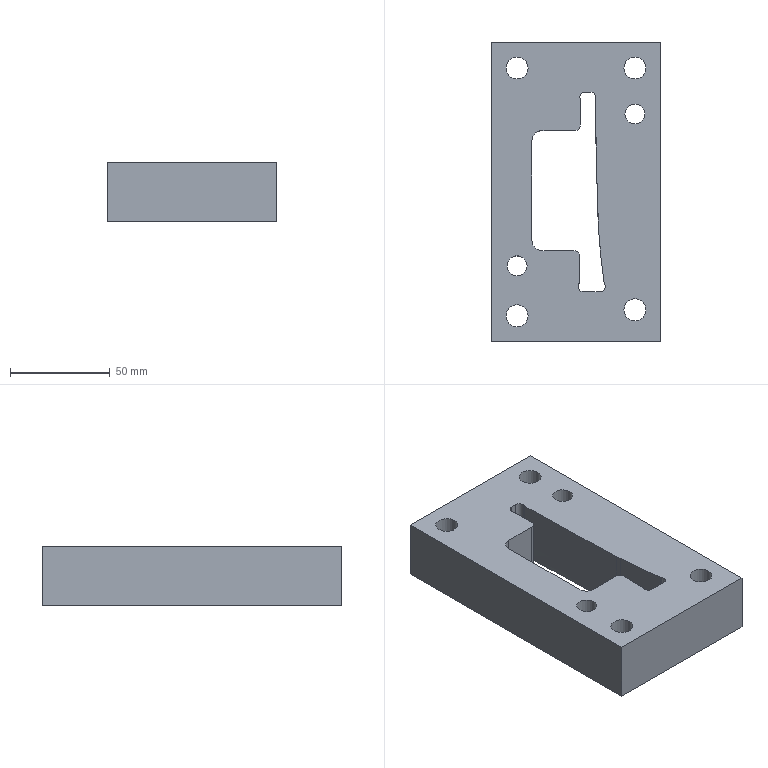Part | STEP file | 202_id726_x_t | 1 solid | 46 faces | box 85 x 150 x 30 mm | volume 287724 mm3 | cylinder 24 | plane 18 | other 4 | commonest cylinder face diameters 5 x8 11 x6 10 x4 17 x4 6 x2